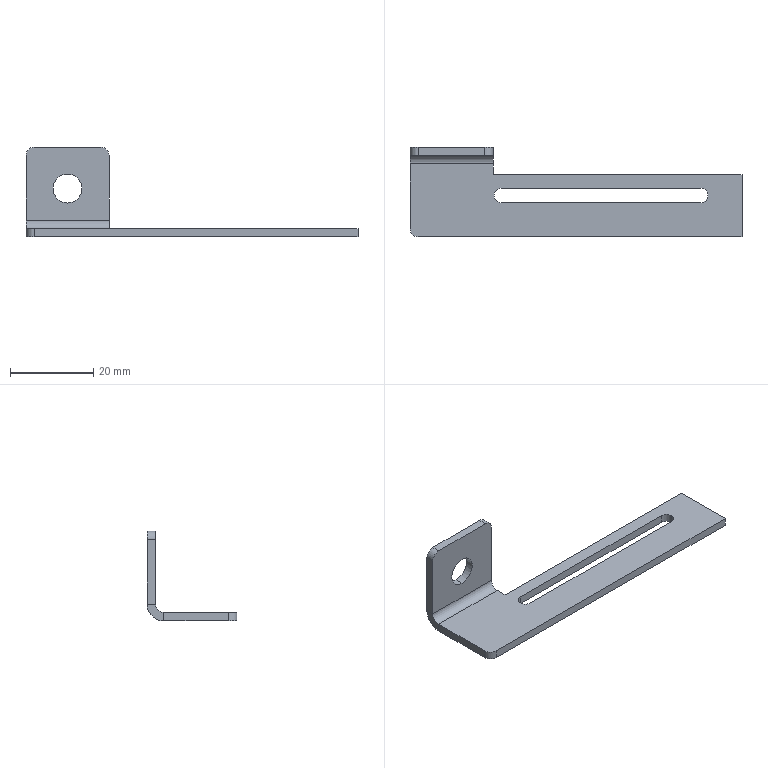Part | STEP file | 601-07-0012 | 1 solid | 26 faces | box 80 x 21.644 x 21.644 mm | volume 2963 mm3 | plane 16 | cylinder 10 | commonest cylinder face diameters 4 x4 3.5 x3 7 x2 8 x1